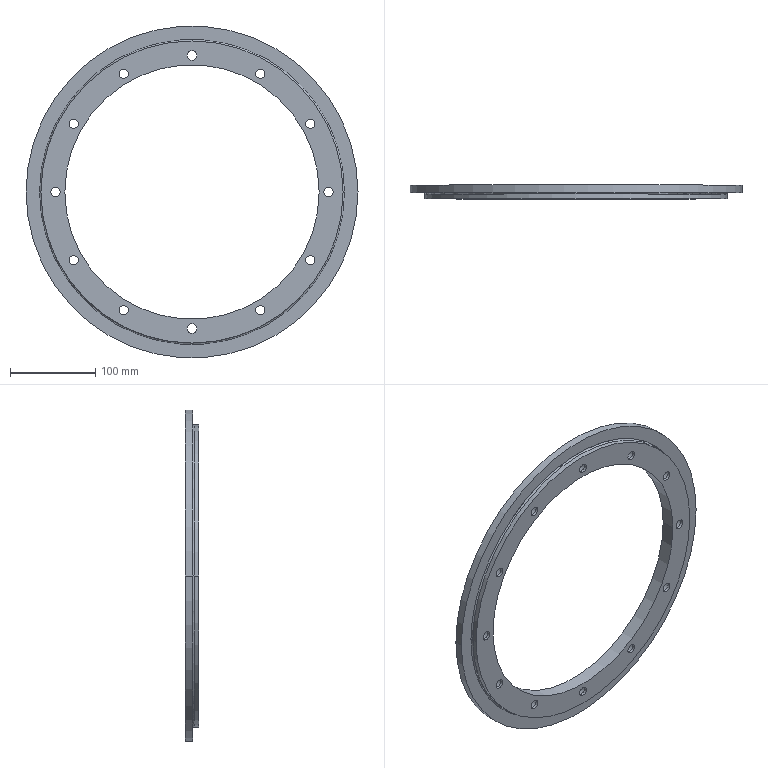Part | SolidWorks | features CirPattern 1, Fillet 1, HoleWzd 1, RefAxis 1, Revolution 1 | 1 solid | 71 faces | box 389 x 16 x 389 mm | volume 600136 mm3 | cylinder 54 | plane 15 | torus 2 | commonest cylinder face diameters 11 x24 18 x24 298 x2 354 x2 389 x2